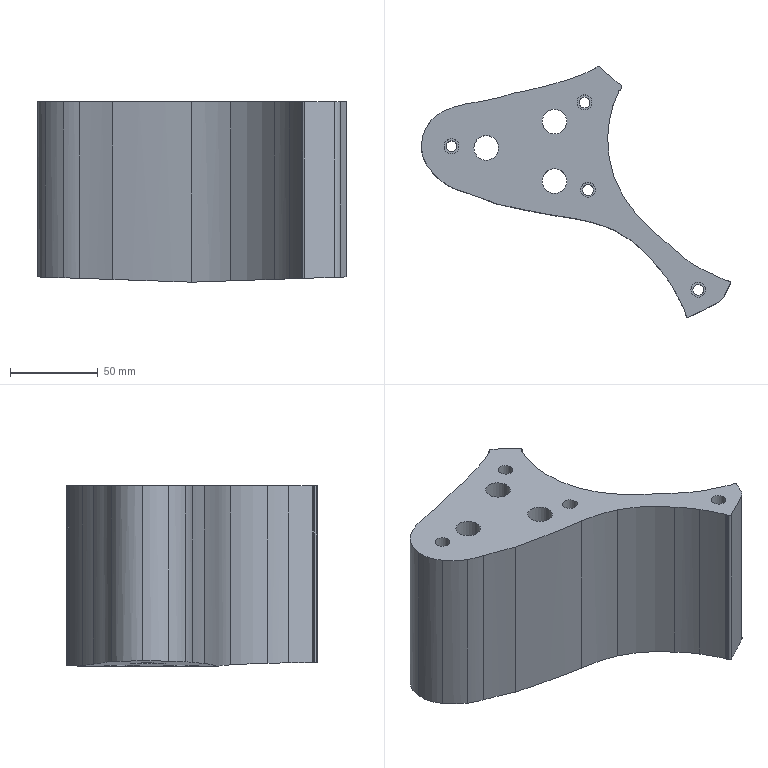Part | NX | features 8 2 | 1 solid | 65 faces | box 176.518 x 143.279 x 103 mm | volume 743357 mm3 | cylinder 48 | plane 15 | spline 2 | commonest cylinder face diameters 2 x10 6.2 x4 8.5 x4 14.1 x3 20 x3 464.919 x2